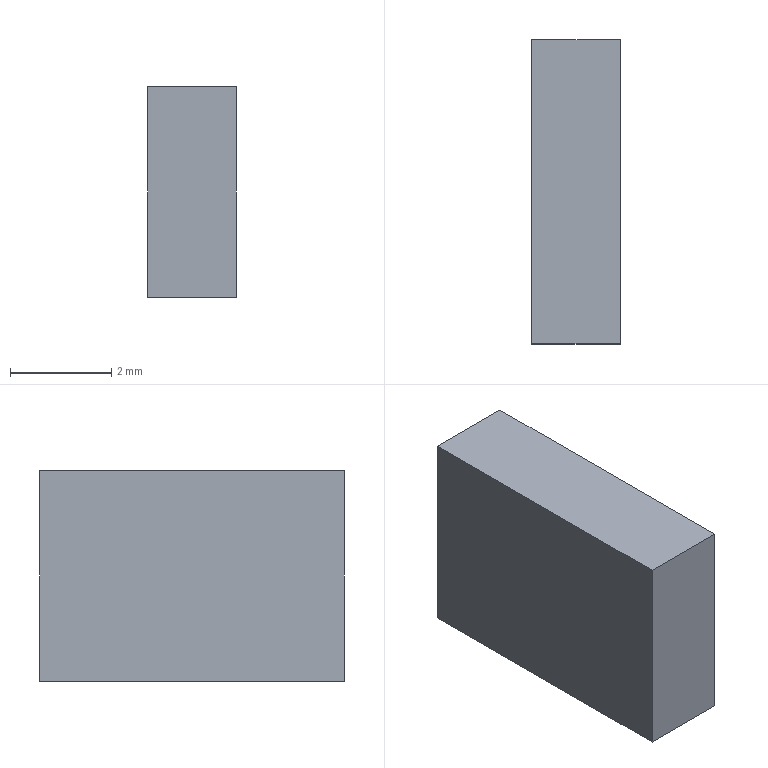Part | STEP file | RJ-USIO-V1_2-220411_65 | 1 solid | 6 faces | box 1.75 x 6 x 4.15 mm | volume 43.575 mm3 | plane 6
STEP:
#1=CARTESIAN_POINT('',(0.,0.,0.));
#2=DIRECTION('',(0.,0.,1.));
#3=DIRECTION('',(1.,0.,0.));
#4=AXIS2_PLACEMENT_3D('',#1,#2,#3);
#5=CARTESIAN_POINT('',(98.15,57.4,4.15));
#6=VERTEX_POINT('',#5);
#7=CARTESIAN_POINT('',(98.15,57.4,0.));
#8=VERTEX_POINT('',#7);
#9=CARTESIAN_POINT('',(98.15,57.4,4.15));
#10=DIRECTION('',(0.,0.,-1.));
#11=VECTOR('',#10,1.);
#12=LINE('',#9,#11);
#13=CARTESIAN_POINT('',(98.15,60.4,2.075));
#14=DIRECTION('',(1.,0.000000012,0.));
#15=DIRECTION('',(0.,0.,-1.));
#16=AXIS2_PLACEMENT_3D('',#13,#14,#15);
#17=PLANE('',#16);
#18=CARTESIAN_POINT('',(-2.075,-3.));
#19=DIRECTION('',(1.,0.));
#20=VECTOR('',#19,1.);
#21=LINE('',#18,#20);
#22=(GEOMETRIC_REPRESENTATION_CONTEXT(2)PARAMETRIC_REPRESENTATION_CONTEXT()REPRESENTATION_CONTEXT('',''));
#23=DEFINITIONAL_REPRESENTATION('',(#21),#22);
#24=PCURVE('',#17,#23);
#25=CARTESIAN_POINT('',(99.025,57.4,2.075));
#26=DIRECTION('',(0.000000012,-1.,0.));
#27=DIRECTION('',(0.,0.,-1.));
#28=AXIS2_PLACEMENT_3D('',#25,#26,#27);
#29=PLANE('',#28);
#30=CARTESIAN_POINT('',(-2.075,-0.875));
#31=DIRECTION('',(1.,0.));
#32=VECTOR('',#31,1.);
#33=LINE('',#30,#32);
#34=(GEOMETRIC_REPRESENTATION_CONTEXT(2)PARAMETRIC_REPRESENTATION_CONTEXT()REPRESENTATION_CONTEXT('',''));
#35=DEFINITIONAL_REPRESENTATION('',(#33),#34);
#36=PCURVE('',#29,#35);
#37=SURFACE_CURVE('',#12,(#24,#36),.PCURVE_S1.);
#38=EDGE_CURVE('',#6,#8,#37,.T.);
#39=ORIENTED_EDGE('',*,*,#38,.T.);
#40=CARTESIAN_POINT('',(98.15,63.4,0.));
#41=VERTEX_POINT('',#40);
#42=CARTESIAN_POINT('',(98.15,57.4,0.));
#43=DIRECTION('',(-0.000000012,1.,0.));
#44=VECTOR('',#43,1.);
#45=LINE('',#42,#44);
#46=CARTESIAN_POINT('',(2.075,-3.));
#47=DIRECTION('',(0.,1.));
#48=VECTOR('',#47,1.);
#49=LINE('',#46,#48);
#50=(GEOMETRIC_REPRESENTATION_CONTEXT(2)PARAMETRIC_REPRESENTATION_CONTEXT()REPRESENTATION_CONTEXT('',''));
#51=DEFINITIONAL_REPRESENTATION('',(#49),#50);
#52=PCURVE('',#17,#51);
#53=CARTESIAN_POINT('',(99.025,60.4,0.));
#54=DIRECTION('',(0.,0.,1.));
#55=DIRECTION('',(-0.000000012,1.,0.));
#56=AXIS2_PLACEMENT_3D('',#53,#54,#55);
#57=PLANE('',#56);
#58=CARTESIAN_POINT('',(-3.,0.875));
#59=DIRECTION('',(1.,0.));
#60=VECTOR('',#59,1.);
#61=LINE('',#58,#60);
#62=(GEOMETRIC_REPRESENTATION_CONTEXT(2)PARAMETRIC_REPRESENTATION_CONTEXT()REPRESENTATION_CONTEXT('',''));
#63=DEFINITIONAL_REPRESENTATION('',(#61),#62);
#64=PCURVE('',#57,#63);
#65=SURFACE_CURVE('',#45,(#52,#64),.PCURVE_S1.);
#66=EDGE_CURVE('',#8,#41,#65,.T.);
#67=ORIENTED_EDGE('',*,*,#66,.T.);
#68=CARTESIAN_POINT('',(98.15,63.4,4.15));
#69=VERTEX_POINT('',#68);
#70=CARTESIAN_POINT('',(98.15,63.4,0.));
#71=DIRECTION('',(0.,0.,1.));
#72=VECTOR('',#71,1.);
#73=LINE('',#70,#72);
#74=CARTESIAN_POINT('',(2.075,3.));
#75=DIRECTION('',(-1.,0.));
#76=VECTOR('',#75,1.);
#77=LINE('',#74,#76);
#78=(GEOMETRIC_REPRESENTATION_CONTEXT(2)PARAMETRIC_REPRESENTATION_CONTEXT()REPRESENTATION_CONTEXT('',''));
#79=DEFINITIONAL_REPRESENTATION('',(#77),#78);
#80=PCURVE('',#17,#79);
#81=CARTESIAN_POINT('',(99.025,63.4,2.075));
#82=DIRECTION('',(0.000000012,-1.,0.));
#83=DIRECTION('',(0.,0.,1.));
#84=AXIS2_PLACEMENT_3D('',#81,#82,#83);
#85=PLANE('',#84);
#86=CARTESIAN_POINT('',(-2.075,0.875));
#87=DIRECTION('',(1.,0.));
#88=VECTOR('',#87,1.);
#89=LINE('',#86,#88);
#90=(GEOMETRIC_REPRESENTATION_CONTEXT(2)PARAMETRIC_REPRESENTATION_CONTEXT()REPRESENTATION_CONTEXT('',''));
#91=DEFINITIONAL_REPRESENTATION('',(#89),#90);
#92=PCURVE('',#85,#91);
#93=SURFACE_CURVE('',#73,(#80,#92),.PCURVE_S1.);
#94=EDGE_CURVE('',#41,#69,#93,.T.);
#95=ORIENTED_EDGE('',*,*,#94,.T.);
#96=CARTESIAN_POINT('',(98.15,63.4,4.15));
#97=DIRECTION('',(0.000000012,-1.,0.));
#98=VECTOR('',#97,1.);
#99=LINE('',#96,#98);
#100=CARTESIAN_POINT('',(-2.075,3.));
#101=DIRECTION('',(0.,-1.));
#102=VECTOR('',#101,1.);
#103=LINE('',#100,#102);
#104=(GEOMETRIC_REPRESENTATION_CONTEXT(2)PARAMETRIC_REPRESENTATION_CONTEXT()REPRESENTATION_CONTEXT('',''));
#105=DEFINITIONAL_REPRESENTATION('',(#103),#104);
#106=PCURVE('',#17,#105);
#107=CARTESIAN_POINT('',(99.025,60.4,4.15));
#108=DIRECTION('',(0.,0.,1.));
#109=DIRECTION('',(-0.000000012,1.,0.));
#110=AXIS2_PLACEMENT_3D('',#107,#108,#109);
#111=PLANE('',#110);
#112=CARTESIAN_POINT('',(3.,0.875));
#113=DIRECTION('',(-1.,0.));
#114=VECTOR('',#113,1.);
#115=LINE('',#112,#114);
#116=(GEOMETRIC_REPRESENTATION_CONTEXT(2)PARAMETRIC_REPRESENTATION_CONTEXT()REPRESENTATION_CONTEXT('',''));
#117=DEFINITIONAL_REPRESENTATION('',(#115),#116);
#118=PCURVE('',#111,#117);
#119=SURFACE_CURVE('',#99,(#106,#118),.PCURVE_S1.);
#120=EDGE_CURVE('',#69,#6,#119,.T.);
#121=ORIENTED_EDGE('',*,*,#120,.T.);
#122=EDGE_LOOP('',(#39,#67,#95,#121));
#123=FACE_BOUND('',#122,.F.);
#124=ADVANCED_FACE('',(#123),#17,.F.);
#125=CARTESIAN_POINT('',(99.9,57.4,4.15));
#126=VERTEX_POINT('',#125);
#127=CARTESIAN_POINT('',(99.9,57.4,0.));
#128=VERTEX_POINT('',#127);
#129=CARTESIAN_POINT('',(99.9,57.4,4.15));
#130=DIRECTION('',(0.,0.,-1.));
#131=VECTOR('',#130,1.);
#132=LINE('',#129,#131);
#133=CARTESIAN_POINT('',(-2.075,0.875));
#134=DIRECTION('',(1.,0.));
#135=VECTOR('',#134,1.);
#136=LINE('',#133,#135);
#137=(GEOMETRIC_REPRESENTATION_CONTEXT(2)PARAMETRIC_REPRESENTATION_CONTEXT()REPRESENTATION_CONTEXT('',''));
#138=DEFINITIONAL_REPRESENTATION('',(#136),#137);
#139=PCURVE('',#29,#138);
#140=CARTESIAN_POINT('',(99.9,60.4,2.075));
#141=DIRECTION('',(1.,0.000000012,0.));
#142=DIRECTION('',(-0.000000012,1.,0.));
#143=AXIS2_PLACEMENT_3D('',#140,#141,#142);
#144=PLANE('',#143);
#145=CARTESIAN_POINT('',(-3.,2.075));
#146=DIRECTION('',(0.,-1.));
#147=VECTOR('',#146,1.);
#148=LINE('',#145,#147);
#149=(GEOMETRIC_REPRESENTATION_CONTEXT(2)PARAMETRIC_REPRESENTATION_CONTEXT()REPRESENTATION_CONTEXT('',''));
#150=DEFINITIONAL_REPRESENTATION('',(#148),#149);
#151=PCURVE('',#144,#150);
#152=SURFACE_CURVE('',#132,(#139,#151),.PCURVE_S1.);
#153=EDGE_CURVE('',#126,#128,#152,.T.);
#154=ORIENTED_EDGE('',*,*,#153,.T.);
#155=CARTESIAN_POINT('',(98.15,57.4,0.));
#156=DIRECTION('',(1.,0.000000012,0.));
#157=VECTOR('',#156,1.);
#158=LINE('',#155,#157);
#159=CARTESIAN_POINT('',(2.075,-0.875));
#160=DIRECTION('',(0.,1.));
#161=VECTOR('',#160,1.);
#162=LINE('',#159,#161);
#163=(GEOMETRIC_REPRESENTATION_CONTEXT(2)PARAMETRIC_REPRESENTATION_CONTEXT()REPRESENTATION_CONTEXT('',''));
#164=DEFINITIONAL_REPRESENTATION('',(#162),#163);
#165=PCURVE('',#29,#164);
#166=CARTESIAN_POINT('',(-3.,0.875));
#167=DIRECTION('',(0.,-1.));
#168=VECTOR('',#167,1.);
#169=LINE('',#166,#168);
#170=(GEOMETRIC_REPRESENTATION_CONTEXT(2)PARAMETRIC_REPRESENTATION_CONTEXT()REPRESENTATION_CONTEXT('',''));
#171=DEFINITIONAL_REPRESENTATION('',(#169),#170);
#172=PCURVE('',#57,#171);
#173=SURFACE_CURVE('',#158,(#165,#172),.PCURVE_S1.);
#174=EDGE_CURVE('',#8,#128,#173,.T.);
#175=ORIENTED_EDGE('',*,*,#174,.F.);
#176=ORIENTED_EDGE('',*,*,#38,.F.);
#177=CARTESIAN_POINT('',(98.15,57.4,4.15));
#178=DIRECTION('',(1.,0.000000012,0.));
#179=VECTOR('',#178,1.);
#180=LINE('',#177,#179);
#181=CARTESIAN_POINT('',(-2.075,-0.875));
#182=DIRECTION('',(0.,1.));
#183=VECTOR('',#182,1.);
#184=LINE('',#181,#183);
#185=(GEOMETRIC_REPRESENTATION_CONTEXT(2)PARAMETRIC_REPRESENTATION_CONTEXT()REPRESENTATION_CONTEXT('',''));
#186=DEFINITIONAL_REPRESENTATION('',(#184),#185);
#187=PCURVE('',#29,#186);
#188=CARTESIAN_POINT('',(-3.,0.875));
#189=DIRECTION('',(0.,-1.));
#190=VECTOR('',#189,1.);
#191=LINE('',#188,#190);
#192=(GEOMETRIC_REPRESENTATION_CONTEXT(2)PARAMETRIC_REPRESENTATION_CONTEXT()REPRESENTATION_CONTEXT('',''));
#193=DEFINITIONAL_REPRESENTATION('',(#191),#192);
#194=PCURVE('',#111,#193);
#195=SURFACE_CURVE('',#180,(#187,#194),.PCURVE_S1.);
#196=EDGE_CURVE('',#6,#126,#195,.T.);
#197=ORIENTED_EDGE('',*,*,#196,.T.);
#198=EDGE_LOOP('',(#154,#175,#176,#197));
#199=FACE_BOUND('',#198,.F.);
#200=ADVANCED_FACE('',(#199),#29,.T.);
#201=CARTESIAN_POINT('',(99.9,63.4,0.));
#202=VERTEX_POINT('',#201);
#203=CARTESIAN_POINT('',(99.9,63.4,4.15));
#204=VERTEX_POINT('',#203);
#205=CARTESIAN_POINT('',(99.9,63.4,0.));
#206=DIRECTION('',(0.,0.,1.));
#207=VECTOR('',#206,1.);
#208=LINE('',#205,#207);
#209=CARTESIAN_POINT('',(3.,-2.075));
#210=DIRECTION('',(0.,1.));
#211=VECTOR('',#210,1.);
#212=LINE('',#209,#211);
#213=(GEOMETRIC_REPRESENTATION_CONTEXT(2)PARAMETRIC_REPRESENTATION_CONTEXT()REPRESENTATION_CONTEXT('',''));
#214=DEFINITIONAL_REPRESENTATION('',(#212),#213);
#215=PCURVE('',#144,#214);
#216=CARTESIAN_POINT('',(-2.075,-0.875));
#217=DIRECTION('',(1.,0.));
#218=VECTOR('',#217,1.);
#219=LINE('',#216,#218);
#220=(GEOMETRIC_REPRESENTATION_CONTEXT(2)PARAMETRIC_REPRESENTATION_CONTEXT()REPRESENTATION_CONTEXT('',''));
#221=DEFINITIONAL_REPRESENTATION('',(#219),#220);
#222=PCURVE('',#85,#221);
#223=SURFACE_CURVE('',#208,(#215,#222),.PCURVE_S1.);
#224=EDGE_CURVE('',#202,#204,#223,.T.);
#225=ORIENTED_EDGE('',*,*,#224,.F.);
#226=CARTESIAN_POINT('',(99.9,57.4,0.));
#227=DIRECTION('',(-0.000000012,1.,0.));
#228=VECTOR('',#227,1.);
#229=LINE('',#226,#228);
#230=CARTESIAN_POINT('',(-3.,-2.075));
#231=DIRECTION('',(1.,0.));
#232=VECTOR('',#231,1.);
#233=LINE('',#230,#232);
#234=(GEOMETRIC_REPRESENTATION_CONTEXT(2)PARAMETRIC_REPRESENTATION_CONTEXT()REPRESENTATION_CONTEXT('',''));
#235=DEFINITIONAL_REPRESENTATION('',(#233),#234);
#236=PCURVE('',#144,#235);
#237=CARTESIAN_POINT('',(-3.,-0.875));
#238=DIRECTION('',(1.,0.));
#239=VECTOR('',#238,1.);
#240=LINE('',#237,#239);
#241=(GEOMETRIC_REPRESENTATION_CONTEXT(2)PARAMETRIC_REPRESENTATION_CONTEXT()REPRESENTATION_CONTEXT('',''));
#242=DEFINITIONAL_REPRESENTATION('',(#240),#241);
#243=PCURVE('',#57,#242);
#244=SURFACE_CURVE('',#229,(#236,#243),.PCURVE_S1.);
#245=EDGE_CURVE('',#128,#202,#244,.T.);
#246=ORIENTED_EDGE('',*,*,#245,.F.);
#247=ORIENTED_EDGE('',*,*,#153,.F.);
#248=CARTESIAN_POINT('',(99.9,57.4,4.15));
#249=DIRECTION('',(-0.000000012,1.,0.));
#250=VECTOR('',#249,1.);
#251=LINE('',#248,#250);
#252=CARTESIAN_POINT('',(-3.,2.075));
#253=DIRECTION('',(1.,0.));
#254=VECTOR('',#253,1.);
#255=LINE('',#252,#254);
#256=(GEOMETRIC_REPRESENTATION_CONTEXT(2)PARAMETRIC_REPRESENTATION_CONTEXT()REPRESENTATION_CONTEXT('',''));
#257=DEFINITIONAL_REPRESENTATION('',(#255),#256);
#258=PCURVE('',#144,#257);
#259=CARTESIAN_POINT('',(-3.,-0.875));
#260=DIRECTION('',(1.,0.));
#261=VECTOR('',#260,1.);
#262=LINE('',#259,#261);
#263=(GEOMETRIC_REPRESENTATION_CONTEXT(2)PARAMETRIC_REPRESENTATION_CONTEXT()REPRESENTATION_CONTEXT('',''));
#264=DEFINITIONAL_REPRESENTATION('',(#262),#263);
#265=PCURVE('',#111,#264);
#266=SURFACE_CURVE('',#251,(#258,#265),.PCURVE_S1.);
#267=EDGE_CURVE('',#126,#204,#266,.T.);
#268=ORIENTED_EDGE('',*,*,#267,.T.);
#269=EDGE_LOOP('',(#225,#246,#247,#268));
#270=FACE_BOUND('',#269,.F.);
#271=ADVANCED_FACE('',(#270),#144,.T.);
#272=ORIENTED_EDGE('',*,*,#94,.F.);
#273=CARTESIAN_POINT('',(99.9,63.4,0.));
#274=DIRECTION('',(-1.,-0.000000012,0.));
#275=VECTOR('',#274,1.);
#276=LINE('',#273,#275);
#277=CARTESIAN_POINT('',(-2.075,-0.875));
#278=DIRECTION('',(0.,1.));
#279=VECTOR('',#278,1.);
#280=LINE('',#277,#279);
#281=(GEOMETRIC_REPRESENTATION_CONTEXT(2)PARAMETRIC_REPRESENTATION_CONTEXT()REPRESENTATION_CONTEXT('',''));
#282=DEFINITIONAL_REPRESENTATION('',(#280),#281);
#283=PCURVE('',#85,#282);
#284=CARTESIAN_POINT('',(3.,-0.875));
#285=DIRECTION('',(0.,1.));
#286=VECTOR('',#285,1.);
#287=LINE('',#284,#286);
#288=(GEOMETRIC_REPRESENTATION_CONTEXT(2)PARAMETRIC_REPRESENTATION_CONTEXT()REPRESENTATION_CONTEXT('',''));
#289=DEFINITIONAL_REPRESENTATION('',(#287),#288);
#290=PCURVE('',#57,#289);
#291=SURFACE_CURVE('',#276,(#283,#290),.PCURVE_S1.);
#292=EDGE_CURVE('',#202,#41,#291,.T.);
#293=ORIENTED_EDGE('',*,*,#292,.F.);
#294=ORIENTED_EDGE('',*,*,#224,.T.);
#295=CARTESIAN_POINT('',(99.9,63.4,4.15));
#296=DIRECTION('',(-1.,-0.000000012,0.));
#297=VECTOR('',#296,1.);
#298=LINE('',#295,#297);
#299=CARTESIAN_POINT('',(2.075,-0.875));
#300=DIRECTION('',(0.,1.));
#301=VECTOR('',#300,1.);
#302=LINE('',#299,#301);
#303=(GEOMETRIC_REPRESENTATION_CONTEXT(2)PARAMETRIC_REPRESENTATION_CONTEXT()REPRESENTATION_CONTEXT('',''));
#304=DEFINITIONAL_REPRESENTATION('',(#302),#303);
#305=PCURVE('',#85,#304);
#306=CARTESIAN_POINT('',(3.,-0.875));
#307=DIRECTION('',(0.,1.));
#308=VECTOR('',#307,1.);
#309=LINE('',#306,#308);
#310=(GEOMETRIC_REPRESENTATION_CONTEXT(2)PARAMETRIC_REPRESENTATION_CONTEXT()REPRESENTATION_CONTEXT('',''));
#311=DEFINITIONAL_REPRESENTATION('',(#309),#310);
#312=PCURVE('',#111,#311);
#313=SURFACE_CURVE('',#298,(#305,#312),.PCURVE_S1.);
#314=EDGE_CURVE('',#204,#69,#313,.T.);
#315=ORIENTED_EDGE('',*,*,#314,.T.);
#316=EDGE_LOOP('',(#272,#293,#294,#315));
#317=FACE_BOUND('',#316,.F.);
#318=ADVANCED_FACE('',(#317),#85,.F.);
#319=ORIENTED_EDGE('',*,*,#245,.T.);
#320=ORIENTED_EDGE('',*,*,#292,.T.);
#321=ORIENTED_EDGE('',*,*,#66,.F.);
#322=ORIENTED_EDGE('',*,*,#174,.T.);
#323=EDGE_LOOP('',(#319,#320,#321,#322));
#324=FACE_BOUND('',#323,.F.);
#325=ADVANCED_FACE('',(#324),#57,.F.);
#326=ORIENTED_EDGE('',*,*,#267,.F.);
#327=ORIENTED_EDGE('',*,*,#196,.F.);
#328=ORIENTED_EDGE('',*,*,#120,.F.);
#329=ORIENTED_EDGE('',*,*,#314,.F.);
#330=EDGE_LOOP('',(#326,#327,#328,#329));
#331=FACE_BOUND('',#330,.F.);
#332=ADVANCED_FACE('',(#331),#111,.T.);
#333=CLOSED_SHELL('',(#124,#200,#271,#318,#325,#332));
#334=MANIFOLD_SOLID_BREP('',#333);
#335=(LENGTH_UNIT()NAMED_UNIT(*)SI_UNIT(.MILLI.,.METRE.));
#336=UNCERTAINTY_MEASURE_WITH_UNIT(LENGTH_MEASURE(0.0000001),#335,'','');
#337=(NAMED_UNIT(*)PLANE_ANGLE_UNIT()SI_UNIT($,.RADIAN.));
#338=(NAMED_UNIT(*)SI_UNIT($,.STERADIAN.)SOLID_ANGLE_UNIT());
#339=(GEOMETRIC_REPRESENTATION_CONTEXT(3)GLOBAL_UNCERTAINTY_ASSIGNED_CONTEXT((#336))GLOBAL_UNIT_ASSIGNED_CONTEXT((#335,#337,#338))REPRESENTATION_CONTEXT('',''));
#340=ADVANCED_BREP_SHAPE_REPRESENTATION('',(#4,#334),#339);